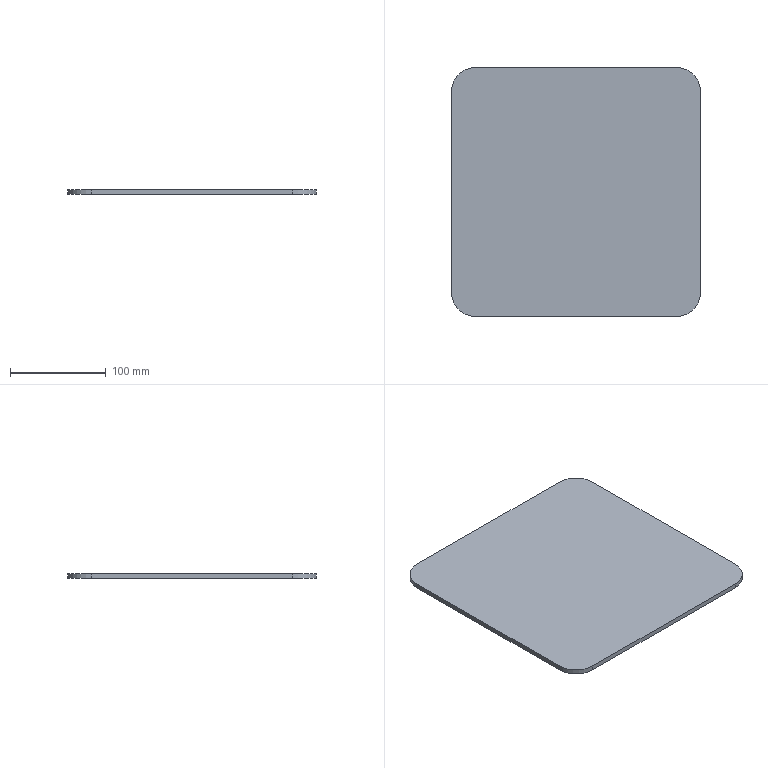Part | SolidWorks | features FlatPattern 1, SMBaseFlange 1, SheetMetal 1 | 1 solid | 10 faces | box 260 x 260 x 5 mm | volume 335317 mm3 | plane 6 | cylinder 4 | commonest cylinder face diameters 50 x4
STEP:
#1=CARTESIAN_POINT('',(-114.544,154.146,0.));
#2=VERTEX_POINT('',#1);
#3=CARTESIAN_POINT('',(-139.544,129.146,0.));
#4=VERTEX_POINT('',#3);
#5=CARTESIAN_POINT('',(-114.544,129.146,0.));
#6=DIRECTION('',(0.,0.,1.));
#7=DIRECTION('',(1.,0.,0.));
#8=AXIS2_PLACEMENT_3D('',#5,#6,#7);
#9=CIRCLE('',#8,25.);
#10=EDGE_CURVE('',#2,#4,#9,.T.);
#11=ORIENTED_EDGE('',*,*,#10,.T.);
#12=CARTESIAN_POINT('',(-139.544,129.146,5.));
#13=VERTEX_POINT('',#12);
#14=CARTESIAN_POINT('',(-139.544,129.146,5.));
#15=DIRECTION('',(0.,0.,-1.));
#16=VECTOR('',#15,1000.);
#17=LINE('',#14,#16);
#18=EDGE_CURVE('',#13,#4,#17,.T.);
#19=ORIENTED_EDGE('',*,*,#18,.F.);
#20=CARTESIAN_POINT('',(-114.544,154.146,5.));
#21=VERTEX_POINT('',#20);
#22=CARTESIAN_POINT('',(-114.544,129.146,5.));
#23=DIRECTION('',(0.,0.,1.));
#24=DIRECTION('',(1.,0.,0.));
#25=AXIS2_PLACEMENT_3D('',#22,#23,#24);
#26=CIRCLE('',#25,25.);
#27=EDGE_CURVE('',#21,#13,#26,.T.);
#28=ORIENTED_EDGE('',*,*,#27,.F.);
#29=CARTESIAN_POINT('',(-114.544,154.146,5.));
#30=DIRECTION('',(0.,0.,-1.));
#31=VECTOR('',#30,1000.);
#32=LINE('',#29,#31);
#33=EDGE_CURVE('',#21,#2,#32,.T.);
#34=ORIENTED_EDGE('',*,*,#33,.T.);
#35=EDGE_LOOP('',(#11,#19,#28,#34));
#36=FACE_OUTER_BOUND('',#35,.T.);
#37=CARTESIAN_POINT('',(-114.544,129.146,5.));
#38=DIRECTION('',(0.,0.,-1.));
#39=DIRECTION('',(-1.,0.,0.));
#40=AXIS2_PLACEMENT_3D('',#37,#38,#39);
#41=CYLINDRICAL_SURFACE('',#40,25.);
#42=ADVANCED_FACE('',(#36),#41,.T.);
#43=CARTESIAN_POINT('',(-139.544,-80.854,0.));
#44=VERTEX_POINT('',#43);
#45=CARTESIAN_POINT('',(-139.544,129.146,0.));
#46=DIRECTION('',(0.,-1.,0.));
#47=VECTOR('',#46,1000.);
#48=LINE('',#45,#47);
#49=EDGE_CURVE('',#4,#44,#48,.T.);
#50=ORIENTED_EDGE('',*,*,#49,.T.);
#51=CARTESIAN_POINT('',(-139.544,-80.854,5.));
#52=VERTEX_POINT('',#51);
#53=CARTESIAN_POINT('',(-139.544,-80.854,5.));
#54=DIRECTION('',(0.,0.,-1.));
#55=VECTOR('',#54,1000.);
#56=LINE('',#53,#55);
#57=EDGE_CURVE('',#52,#44,#56,.T.);
#58=ORIENTED_EDGE('',*,*,#57,.F.);
#59=CARTESIAN_POINT('',(-139.544,129.146,5.));
#60=DIRECTION('',(0.,-1.,0.));
#61=VECTOR('',#60,1000.);
#62=LINE('',#59,#61);
#63=EDGE_CURVE('',#13,#52,#62,.T.);
#64=ORIENTED_EDGE('',*,*,#63,.F.);
#65=ORIENTED_EDGE('',*,*,#18,.T.);
#66=EDGE_LOOP('',(#50,#58,#64,#65));
#67=FACE_OUTER_BOUND('',#66,.T.);
#68=CARTESIAN_POINT('',(-139.544,129.146,5.));
#69=DIRECTION('',(1.,0.,0.));
#70=DIRECTION('',(0.,1.,0.));
#71=AXIS2_PLACEMENT_3D('',#68,#69,#70);
#72=PLANE('',#71);
#73=ADVANCED_FACE('',(#67),#72,.F.);
#74=CARTESIAN_POINT('',(-114.544,-105.854,0.));
#75=VERTEX_POINT('',#74);
#76=CARTESIAN_POINT('',(-114.544,-80.854,0.));
#77=DIRECTION('',(0.,0.,1.));
#78=DIRECTION('',(-1.,0.,0.));
#79=AXIS2_PLACEMENT_3D('',#76,#77,#78);
#80=CIRCLE('',#79,25.);
#81=EDGE_CURVE('',#44,#75,#80,.T.);
#82=ORIENTED_EDGE('',*,*,#81,.T.);
#83=CARTESIAN_POINT('',(-114.544,-105.854,5.));
#84=VERTEX_POINT('',#83);
#85=CARTESIAN_POINT('',(-114.544,-105.854,5.));
#86=DIRECTION('',(0.,0.,-1.));
#87=VECTOR('',#86,1000.);
#88=LINE('',#85,#87);
#89=EDGE_CURVE('',#84,#75,#88,.T.);
#90=ORIENTED_EDGE('',*,*,#89,.F.);
#91=CARTESIAN_POINT('',(-114.544,-80.854,5.));
#92=DIRECTION('',(0.,0.,1.));
#93=DIRECTION('',(-1.,0.,0.));
#94=AXIS2_PLACEMENT_3D('',#91,#92,#93);
#95=CIRCLE('',#94,25.);
#96=EDGE_CURVE('',#52,#84,#95,.T.);
#97=ORIENTED_EDGE('',*,*,#96,.F.);
#98=ORIENTED_EDGE('',*,*,#57,.T.);
#99=EDGE_LOOP('',(#82,#90,#97,#98));
#100=FACE_OUTER_BOUND('',#99,.T.);
#101=CARTESIAN_POINT('',(-114.544,-80.854,5.));
#102=DIRECTION('',(0.,0.,-1.));
#103=DIRECTION('',(-1.,0.,0.));
#104=AXIS2_PLACEMENT_3D('',#101,#102,#103);
#105=CYLINDRICAL_SURFACE('',#104,25.);
#106=ADVANCED_FACE('',(#100),#105,.T.);
#107=CARTESIAN_POINT('',(95.456,-105.854,0.));
#108=VERTEX_POINT('',#107);
#109=CARTESIAN_POINT('',(95.456,-105.854,0.));
#110=DIRECTION('',(1.,0.,0.));
#111=VECTOR('',#110,1000.);
#112=LINE('',#109,#111);
#113=EDGE_CURVE('',#75,#108,#112,.T.);
#114=ORIENTED_EDGE('',*,*,#113,.T.);
#115=CARTESIAN_POINT('',(95.456,-105.854,5.));
#116=VERTEX_POINT('',#115);
#117=CARTESIAN_POINT('',(95.456,-105.854,5.));
#118=DIRECTION('',(0.,0.,-1.));
#119=VECTOR('',#118,1000.);
#120=LINE('',#117,#119);
#121=EDGE_CURVE('',#116,#108,#120,.T.);
#122=ORIENTED_EDGE('',*,*,#121,.F.);
#123=CARTESIAN_POINT('',(95.456,-105.854,5.));
#124=DIRECTION('',(1.,0.,0.));
#125=VECTOR('',#124,1000.);
#126=LINE('',#123,#125);
#127=EDGE_CURVE('',#84,#116,#126,.T.);
#128=ORIENTED_EDGE('',*,*,#127,.F.);
#129=ORIENTED_EDGE('',*,*,#89,.T.);
#130=EDGE_LOOP('',(#114,#122,#128,#129));
#131=FACE_OUTER_BOUND('',#130,.T.);
#132=CARTESIAN_POINT('',(95.456,-105.854,5.));
#133=DIRECTION('',(0.,1.,0.));
#134=DIRECTION('',(-1.,0.,0.));
#135=AXIS2_PLACEMENT_3D('',#132,#133,#134);
#136=PLANE('',#135);
#137=ADVANCED_FACE('',(#131),#136,.F.);
#138=CARTESIAN_POINT('',(120.456,-80.854,0.));
#139=VERTEX_POINT('',#138);
#140=CARTESIAN_POINT('',(95.456,-80.854,0.));
#141=DIRECTION('',(0.,0.,1.));
#142=DIRECTION('',(-1.,0.,0.));
#143=AXIS2_PLACEMENT_3D('',#140,#141,#142);
#144=CIRCLE('',#143,25.);
#145=EDGE_CURVE('',#108,#139,#144,.T.);
#146=ORIENTED_EDGE('',*,*,#145,.T.);
#147=CARTESIAN_POINT('',(120.456,-80.854,5.));
#148=VERTEX_POINT('',#147);
#149=CARTESIAN_POINT('',(120.456,-80.854,5.));
#150=DIRECTION('',(0.,0.,-1.));
#151=VECTOR('',#150,1000.);
#152=LINE('',#149,#151);
#153=EDGE_CURVE('',#148,#139,#152,.T.);
#154=ORIENTED_EDGE('',*,*,#153,.F.);
#155=CARTESIAN_POINT('',(95.456,-80.854,5.));
#156=DIRECTION('',(0.,0.,1.));
#157=DIRECTION('',(-1.,0.,0.));
#158=AXIS2_PLACEMENT_3D('',#155,#156,#157);
#159=CIRCLE('',#158,25.);
#160=EDGE_CURVE('',#116,#148,#159,.T.);
#161=ORIENTED_EDGE('',*,*,#160,.F.);
#162=ORIENTED_EDGE('',*,*,#121,.T.);
#163=EDGE_LOOP('',(#146,#154,#161,#162));
#164=FACE_OUTER_BOUND('',#163,.T.);
#165=CARTESIAN_POINT('',(95.456,-80.854,5.));
#166=DIRECTION('',(0.,0.,-1.));
#167=DIRECTION('',(-1.,0.,0.));
#168=AXIS2_PLACEMENT_3D('',#165,#166,#167);
#169=CYLINDRICAL_SURFACE('',#168,25.);
#170=ADVANCED_FACE('',(#164),#169,.T.);
#171=CARTESIAN_POINT('',(120.456,129.146,0.));
#172=VERTEX_POINT('',#171);
#173=CARTESIAN_POINT('',(120.456,129.146,0.));
#174=DIRECTION('',(0.,1.,0.));
#175=VECTOR('',#174,1000.);
#176=LINE('',#173,#175);
#177=EDGE_CURVE('',#139,#172,#176,.T.);
#178=ORIENTED_EDGE('',*,*,#177,.T.);
#179=CARTESIAN_POINT('',(120.456,129.146,5.));
#180=VERTEX_POINT('',#179);
#181=CARTESIAN_POINT('',(120.456,129.146,5.));
#182=DIRECTION('',(0.,0.,-1.));
#183=VECTOR('',#182,1000.);
#184=LINE('',#181,#183);
#185=EDGE_CURVE('',#180,#172,#184,.T.);
#186=ORIENTED_EDGE('',*,*,#185,.F.);
#187=CARTESIAN_POINT('',(120.456,129.146,5.));
#188=DIRECTION('',(0.,1.,0.));
#189=VECTOR('',#188,1000.);
#190=LINE('',#187,#189);
#191=EDGE_CURVE('',#148,#180,#190,.T.);
#192=ORIENTED_EDGE('',*,*,#191,.F.);
#193=ORIENTED_EDGE('',*,*,#153,.T.);
#194=EDGE_LOOP('',(#178,#186,#192,#193));
#195=FACE_OUTER_BOUND('',#194,.T.);
#196=CARTESIAN_POINT('',(120.456,129.146,5.));
#197=DIRECTION('',(-1.,0.,0.));
#198=DIRECTION('',(0.,0.,1.));
#199=AXIS2_PLACEMENT_3D('',#196,#197,#198);
#200=PLANE('',#199);
#201=ADVANCED_FACE('',(#195),#200,.F.);
#202=CARTESIAN_POINT('',(95.456,154.146,0.));
#203=VERTEX_POINT('',#202);
#204=CARTESIAN_POINT('',(95.456,129.146,0.));
#205=DIRECTION('',(0.,0.,1.));
#206=DIRECTION('',(-1.,0.,0.));
#207=AXIS2_PLACEMENT_3D('',#204,#205,#206);
#208=CIRCLE('',#207,25.);
#209=EDGE_CURVE('',#172,#203,#208,.T.);
#210=ORIENTED_EDGE('',*,*,#209,.T.);
#211=CARTESIAN_POINT('',(95.456,154.146,5.));
#212=VERTEX_POINT('',#211);
#213=CARTESIAN_POINT('',(95.456,154.146,5.));
#214=DIRECTION('',(0.,0.,-1.));
#215=VECTOR('',#214,1000.);
#216=LINE('',#213,#215);
#217=EDGE_CURVE('',#212,#203,#216,.T.);
#218=ORIENTED_EDGE('',*,*,#217,.F.);
#219=CARTESIAN_POINT('',(95.456,129.146,5.));
#220=DIRECTION('',(0.,0.,1.));
#221=DIRECTION('',(-1.,0.,0.));
#222=AXIS2_PLACEMENT_3D('',#219,#220,#221);
#223=CIRCLE('',#222,25.);
#224=EDGE_CURVE('',#180,#212,#223,.T.);
#225=ORIENTED_EDGE('',*,*,#224,.F.);
#226=ORIENTED_EDGE('',*,*,#185,.T.);
#227=EDGE_LOOP('',(#210,#218,#225,#226));
#228=FACE_OUTER_BOUND('',#227,.T.);
#229=CARTESIAN_POINT('',(95.456,129.146,5.));
#230=DIRECTION('',(0.,0.,-1.));
#231=DIRECTION('',(-1.,0.,0.));
#232=AXIS2_PLACEMENT_3D('',#229,#230,#231);
#233=CYLINDRICAL_SURFACE('',#232,25.);
#234=ADVANCED_FACE('',(#228),#233,.T.);
#235=CARTESIAN_POINT('',(95.456,154.146,0.));
#236=DIRECTION('',(-1.,0.,0.));
#237=VECTOR('',#236,1000.);
#238=LINE('',#235,#237);
#239=EDGE_CURVE('',#203,#2,#238,.T.);
#240=ORIENTED_EDGE('',*,*,#239,.T.);
#241=ORIENTED_EDGE('',*,*,#33,.F.);
#242=CARTESIAN_POINT('',(95.456,154.146,5.));
#243=DIRECTION('',(-1.,0.,0.));
#244=VECTOR('',#243,1000.);
#245=LINE('',#242,#244);
#246=EDGE_CURVE('',#212,#21,#245,.T.);
#247=ORIENTED_EDGE('',*,*,#246,.F.);
#248=ORIENTED_EDGE('',*,*,#217,.T.);
#249=EDGE_LOOP('',(#240,#241,#247,#248));
#250=FACE_OUTER_BOUND('',#249,.T.);
#251=CARTESIAN_POINT('',(95.456,154.146,5.));
#252=DIRECTION('',(0.,-1.,0.));
#253=DIRECTION('',(1.,0.,0.));
#254=AXIS2_PLACEMENT_3D('',#251,#252,#253);
#255=PLANE('',#254);
#256=ADVANCED_FACE('',(#250),#255,.F.);
#257=ORIENTED_EDGE('',*,*,#27,.T.);
#258=ORIENTED_EDGE('',*,*,#63,.T.);
#259=ORIENTED_EDGE('',*,*,#96,.T.);
#260=ORIENTED_EDGE('',*,*,#127,.T.);
#261=ORIENTED_EDGE('',*,*,#160,.T.);
#262=ORIENTED_EDGE('',*,*,#191,.T.);
#263=ORIENTED_EDGE('',*,*,#224,.T.);
#264=ORIENTED_EDGE('',*,*,#246,.T.);
#265=EDGE_LOOP('',(#257,#258,#259,#260,#261,#262,#263,#264));
#266=FACE_OUTER_BOUND('',#265,.T.);
#267=CARTESIAN_POINT('',(-114.544,129.146,5.));
#268=DIRECTION('',(0.,0.,1.));
#269=DIRECTION('',(1.,0.,0.));
#270=AXIS2_PLACEMENT_3D('',#267,#268,#269);
#271=PLANE('',#270);
#272=ADVANCED_FACE('',(#266),#271,.T.);
#273=ORIENTED_EDGE('',*,*,#10,.F.);
#274=ORIENTED_EDGE('',*,*,#239,.F.);
#275=ORIENTED_EDGE('',*,*,#209,.F.);
#276=ORIENTED_EDGE('',*,*,#177,.F.);
#277=ORIENTED_EDGE('',*,*,#145,.F.);
#278=ORIENTED_EDGE('',*,*,#113,.F.);
#279=ORIENTED_EDGE('',*,*,#81,.F.);
#280=ORIENTED_EDGE('',*,*,#49,.F.);
#281=EDGE_LOOP('',(#273,#274,#275,#276,#277,#278,#279,#280));
#282=FACE_OUTER_BOUND('',#281,.T.);
#283=CARTESIAN_POINT('',(-114.544,129.146,0.));
#284=DIRECTION('',(0.,0.,1.));
#285=DIRECTION('',(1.,0.,0.));
#286=AXIS2_PLACEMENT_3D('',#283,#284,#285);
#287=PLANE('',#286);
#288=ADVANCED_FACE('',(#282),#287,.F.);
#289=CLOSED_SHELL('',(#42,#73,#106,#137,#170,#201,#234,#256,#272,#288));
#290=MANIFOLD_SOLID_BREP('',#289);
#291=CARTESIAN_POINT('',(0.,0.,0.));
#292=DIRECTION('',(0.,0.,1.));
#293=DIRECTION('',(1.,0.,0.));
#294=AXIS2_PLACEMENT_3D('',#291,#292,#293);
#295=(LENGTH_UNIT()NAMED_UNIT(*)SI_UNIT(.MILLI.,.METRE.));
#296=UNCERTAINTY_MEASURE_WITH_UNIT(LENGTH_MEASURE(0.00001),#295,'','');
#297=(NAMED_UNIT(*)PLANE_ANGLE_UNIT()SI_UNIT($,.RADIAN.));
#298=(NAMED_UNIT(*)SI_UNIT($,.STERADIAN.)SOLID_ANGLE_UNIT());
#299=(GEOMETRIC_REPRESENTATION_CONTEXT(3)GLOBAL_UNCERTAINTY_ASSIGNED_CONTEXT((#296))GLOBAL_UNIT_ASSIGNED_CONTEXT((#295,#297,#298))REPRESENTATION_CONTEXT('',''));
#300=ADVANCED_BREP_SHAPE_REPRESENTATION('',(#290,#294),#299);